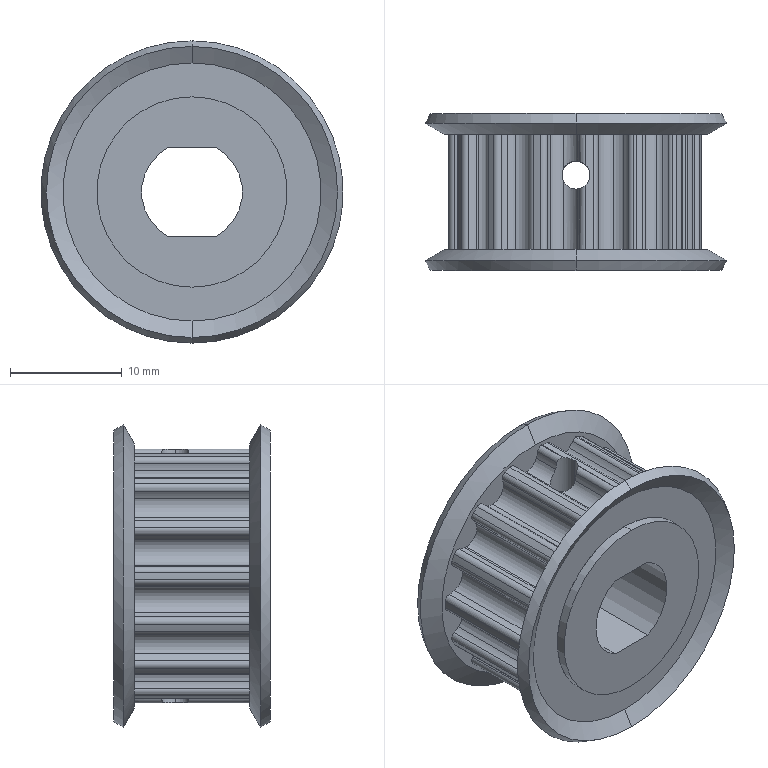Part | NX | features BREP 1 | 1 solid | 151 faces | box 27 x 14 x 27 mm | volume 4073 mm3 | cylinder 125 | cone 16 | plane 10 | commonest cylinder face diameters 1.02 x42 5.08 x33 2.74 x21 22.73 x15 17 x8 2.5 x4